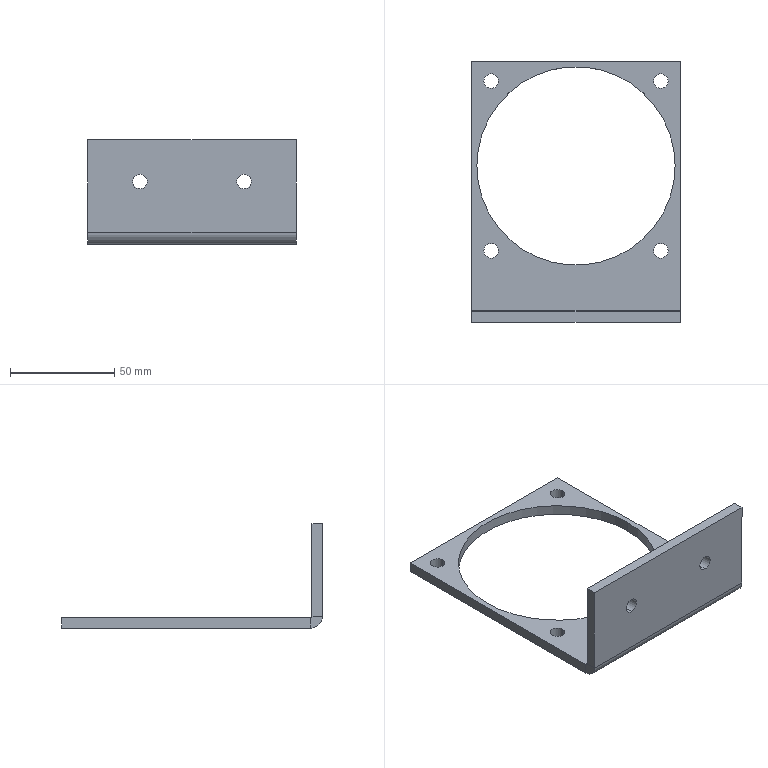Part | SolidWorks | features Cut 1, EdgeFlange 1, FlatPattern 1, ICE 1, SMBaseFlange 1, SheetMetal 1 | 1 solid | 28 faces | box 100 x 125 x 50 mm | volume 47710 mm3 | cylinder 16 | plane 12 | commonest cylinder face diameters 7 x12 95 x2 1.473 x1 11.473 x1
STEP:
#1=CARTESIAN_POINT('',(37.159,53.159,-5.));
#2=VERTEX_POINT('',#1);
#3=CARTESIAN_POINT('',(44.159,53.159,-5.));
#4=VERTEX_POINT('',#3);
#5=CARTESIAN_POINT('',(40.659,53.159,-5.));
#6=DIRECTION('',(0.,0.,1.));
#7=DIRECTION('',(1.,0.,0.));
#8=AXIS2_PLACEMENT_3D('',#5,#6,#7);
#9=CIRCLE('',#8,3.5);
#10=EDGE_CURVE('',#2,#4,#9,.T.);
#11=ORIENTED_EDGE('',*,*,#10,.F.);
#12=CARTESIAN_POINT('',(37.159,53.159,0.));
#13=VERTEX_POINT('',#12);
#14=CARTESIAN_POINT('',(37.159,53.159,-10.));
#15=DIRECTION('',(0.,0.,1.));
#16=VECTOR('',#15,1000.);
#17=LINE('',#14,#16);
#18=EDGE_CURVE('',#2,#13,#17,.T.);
#19=ORIENTED_EDGE('',*,*,#18,.T.);
#20=CARTESIAN_POINT('',(44.159,53.159,0.));
#21=VERTEX_POINT('',#20);
#22=CARTESIAN_POINT('',(40.659,53.159,0.));
#23=DIRECTION('',(0.,0.,1.));
#24=DIRECTION('',(1.,0.,0.));
#25=AXIS2_PLACEMENT_3D('',#22,#23,#24);
#26=CIRCLE('',#25,3.5);
#27=EDGE_CURVE('',#13,#21,#26,.T.);
#28=ORIENTED_EDGE('',*,*,#27,.T.);
#29=CARTESIAN_POINT('',(44.159,53.159,-10.));
#30=DIRECTION('',(0.,0.,1.));
#31=VECTOR('',#30,1000.);
#32=LINE('',#29,#31);
#33=EDGE_CURVE('',#4,#21,#32,.T.);
#34=ORIENTED_EDGE('',*,*,#33,.F.);
#35=EDGE_LOOP('',(#11,#19,#28,#34));
#36=FACE_OUTER_BOUND('',#35,.T.);
#37=CARTESIAN_POINT('',(40.659,53.159,-10.));
#38=DIRECTION('',(0.,0.,1.));
#39=DIRECTION('',(1.,0.,0.));
#40=AXIS2_PLACEMENT_3D('',#37,#38,#39);
#41=CYLINDRICAL_SURFACE('',#40,3.5);
#42=ADVANCED_FACE('',(#36),#41,.F.);
#43=CARTESIAN_POINT('',(37.159,-28.159,-5.));
#44=VERTEX_POINT('',#43);
#45=CARTESIAN_POINT('',(44.159,-28.159,-5.));
#46=VERTEX_POINT('',#45);
#47=CARTESIAN_POINT('',(40.659,-28.159,-5.));
#48=DIRECTION('',(0.,0.,1.));
#49=DIRECTION('',(1.,0.,0.));
#50=AXIS2_PLACEMENT_3D('',#47,#48,#49);
#51=CIRCLE('',#50,3.5);
#52=EDGE_CURVE('',#44,#46,#51,.T.);
#53=ORIENTED_EDGE('',*,*,#52,.F.);
#54=CARTESIAN_POINT('',(37.159,-28.159,0.));
#55=VERTEX_POINT('',#54);
#56=CARTESIAN_POINT('',(37.159,-28.159,-10.));
#57=DIRECTION('',(0.,0.,1.));
#58=VECTOR('',#57,1000.);
#59=LINE('',#56,#58);
#60=EDGE_CURVE('',#44,#55,#59,.T.);
#61=ORIENTED_EDGE('',*,*,#60,.T.);
#62=CARTESIAN_POINT('',(44.159,-28.159,0.));
#63=VERTEX_POINT('',#62);
#64=CARTESIAN_POINT('',(40.659,-28.159,0.));
#65=DIRECTION('',(0.,0.,1.));
#66=DIRECTION('',(1.,0.,0.));
#67=AXIS2_PLACEMENT_3D('',#64,#65,#66);
#68=CIRCLE('',#67,3.5);
#69=EDGE_CURVE('',#55,#63,#68,.T.);
#70=ORIENTED_EDGE('',*,*,#69,.T.);
#71=CARTESIAN_POINT('',(44.159,-28.159,-10.));
#72=DIRECTION('',(0.,0.,1.));
#73=VECTOR('',#72,1000.);
#74=LINE('',#71,#73);
#75=EDGE_CURVE('',#46,#63,#74,.T.);
#76=ORIENTED_EDGE('',*,*,#75,.F.);
#77=EDGE_LOOP('',(#53,#61,#70,#76));
#78=FACE_OUTER_BOUND('',#77,.T.);
#79=CARTESIAN_POINT('',(40.659,-28.159,-10.));
#80=DIRECTION('',(0.,0.,1.));
#81=DIRECTION('',(1.,0.,0.));
#82=AXIS2_PLACEMENT_3D('',#79,#80,#81);
#83=CYLINDRICAL_SURFACE('',#82,3.5);
#84=ADVANCED_FACE('',(#78),#83,.F.);
#85=CARTESIAN_POINT('',(-44.159,-28.159,-5.));
#86=VERTEX_POINT('',#85);
#87=CARTESIAN_POINT('',(-37.159,-28.159,-5.));
#88=VERTEX_POINT('',#87);
#89=CARTESIAN_POINT('',(-40.659,-28.159,-5.));
#90=DIRECTION('',(0.,0.,1.));
#91=DIRECTION('',(1.,0.,0.));
#92=AXIS2_PLACEMENT_3D('',#89,#90,#91);
#93=CIRCLE('',#92,3.5);
#94=EDGE_CURVE('',#86,#88,#93,.T.);
#95=ORIENTED_EDGE('',*,*,#94,.F.);
#96=CARTESIAN_POINT('',(-44.159,-28.159,0.));
#97=VERTEX_POINT('',#96);
#98=CARTESIAN_POINT('',(-44.159,-28.159,-10.));
#99=DIRECTION('',(0.,0.,1.));
#100=VECTOR('',#99,1000.);
#101=LINE('',#98,#100);
#102=EDGE_CURVE('',#86,#97,#101,.T.);
#103=ORIENTED_EDGE('',*,*,#102,.T.);
#104=CARTESIAN_POINT('',(-37.159,-28.159,0.));
#105=VERTEX_POINT('',#104);
#106=CARTESIAN_POINT('',(-40.659,-28.159,0.));
#107=DIRECTION('',(0.,0.,1.));
#108=DIRECTION('',(1.,0.,0.));
#109=AXIS2_PLACEMENT_3D('',#106,#107,#108);
#110=CIRCLE('',#109,3.5);
#111=EDGE_CURVE('',#97,#105,#110,.T.);
#112=ORIENTED_EDGE('',*,*,#111,.T.);
#113=CARTESIAN_POINT('',(-37.159,-28.159,-10.));
#114=DIRECTION('',(0.,0.,1.));
#115=VECTOR('',#114,1000.);
#116=LINE('',#113,#115);
#117=EDGE_CURVE('',#88,#105,#116,.T.);
#118=ORIENTED_EDGE('',*,*,#117,.F.);
#119=EDGE_LOOP('',(#95,#103,#112,#118));
#120=FACE_OUTER_BOUND('',#119,.T.);
#121=CARTESIAN_POINT('',(-40.659,-28.159,-10.));
#122=DIRECTION('',(0.,0.,1.));
#123=DIRECTION('',(1.,0.,0.));
#124=AXIS2_PLACEMENT_3D('',#121,#122,#123);
#125=CYLINDRICAL_SURFACE('',#124,3.5);
#126=ADVANCED_FACE('',(#120),#125,.F.);
#127=CARTESIAN_POINT('',(-44.159,53.159,-5.));
#128=VERTEX_POINT('',#127);
#129=CARTESIAN_POINT('',(-37.159,53.159,-5.));
#130=VERTEX_POINT('',#129);
#131=CARTESIAN_POINT('',(-40.659,53.159,-5.));
#132=DIRECTION('',(0.,0.,1.));
#133=DIRECTION('',(1.,0.,0.));
#134=AXIS2_PLACEMENT_3D('',#131,#132,#133);
#135=CIRCLE('',#134,3.5);
#136=EDGE_CURVE('',#128,#130,#135,.T.);
#137=ORIENTED_EDGE('',*,*,#136,.F.);
#138=CARTESIAN_POINT('',(-44.159,53.159,0.));
#139=VERTEX_POINT('',#138);
#140=CARTESIAN_POINT('',(-44.159,53.159,-10.));
#141=DIRECTION('',(0.,0.,1.));
#142=VECTOR('',#141,1000.);
#143=LINE('',#140,#142);
#144=EDGE_CURVE('',#128,#139,#143,.T.);
#145=ORIENTED_EDGE('',*,*,#144,.T.);
#146=CARTESIAN_POINT('',(-37.159,53.159,0.));
#147=VERTEX_POINT('',#146);
#148=CARTESIAN_POINT('',(-40.659,53.159,0.));
#149=DIRECTION('',(0.,0.,1.));
#150=DIRECTION('',(1.,0.,0.));
#151=AXIS2_PLACEMENT_3D('',#148,#149,#150);
#152=CIRCLE('',#151,3.5);
#153=EDGE_CURVE('',#139,#147,#152,.T.);
#154=ORIENTED_EDGE('',*,*,#153,.T.);
#155=CARTESIAN_POINT('',(-37.159,53.159,-10.));
#156=DIRECTION('',(0.,0.,1.));
#157=VECTOR('',#156,1000.);
#158=LINE('',#155,#157);
#159=EDGE_CURVE('',#130,#147,#158,.T.);
#160=ORIENTED_EDGE('',*,*,#159,.F.);
#161=EDGE_LOOP('',(#137,#145,#154,#160));
#162=FACE_OUTER_BOUND('',#161,.T.);
#163=CARTESIAN_POINT('',(-40.659,53.159,-10.));
#164=DIRECTION('',(0.,0.,1.));
#165=DIRECTION('',(1.,0.,0.));
#166=AXIS2_PLACEMENT_3D('',#163,#164,#165);
#167=CYLINDRICAL_SURFACE('',#166,3.5);
#168=ADVANCED_FACE('',(#162),#167,.F.);
#169=CARTESIAN_POINT('',(-47.5,12.5,-5.));
#170=VERTEX_POINT('',#169);
#171=CARTESIAN_POINT('',(47.5,12.5,-5.));
#172=VERTEX_POINT('',#171);
#173=CARTESIAN_POINT('',(0.,12.5,-5.));
#174=DIRECTION('',(0.,0.,1.));
#175=DIRECTION('',(1.,0.,0.));
#176=AXIS2_PLACEMENT_3D('',#173,#174,#175);
#177=CIRCLE('',#176,47.5);
#178=EDGE_CURVE('',#170,#172,#177,.T.);
#179=ORIENTED_EDGE('',*,*,#178,.F.);
#180=CARTESIAN_POINT('',(-47.5,12.5,0.));
#181=VERTEX_POINT('',#180);
#182=CARTESIAN_POINT('',(-47.5,12.5,-10.));
#183=DIRECTION('',(0.,0.,1.));
#184=VECTOR('',#183,1000.);
#185=LINE('',#182,#184);
#186=EDGE_CURVE('',#170,#181,#185,.T.);
#187=ORIENTED_EDGE('',*,*,#186,.T.);
#188=CARTESIAN_POINT('',(47.5,12.5,0.));
#189=VERTEX_POINT('',#188);
#190=CARTESIAN_POINT('',(0.,12.5,0.));
#191=DIRECTION('',(0.,0.,1.));
#192=DIRECTION('',(1.,0.,0.));
#193=AXIS2_PLACEMENT_3D('',#190,#191,#192);
#194=CIRCLE('',#193,47.5);
#195=EDGE_CURVE('',#181,#189,#194,.T.);
#196=ORIENTED_EDGE('',*,*,#195,.T.);
#197=CARTESIAN_POINT('',(47.5,12.5,-10.));
#198=DIRECTION('',(0.,0.,1.));
#199=VECTOR('',#198,1000.);
#200=LINE('',#197,#199);
#201=EDGE_CURVE('',#172,#189,#200,.T.);
#202=ORIENTED_EDGE('',*,*,#201,.F.);
#203=EDGE_LOOP('',(#179,#187,#196,#202));
#204=FACE_OUTER_BOUND('',#203,.T.);
#205=CARTESIAN_POINT('',(0.,12.5,-10.));
#206=DIRECTION('',(0.,0.,1.));
#207=DIRECTION('',(1.,0.,0.));
#208=AXIS2_PLACEMENT_3D('',#205,#206,#207);
#209=CYLINDRICAL_SURFACE('',#208,47.5);
#210=ADVANCED_FACE('',(#204),#209,.F.);
#211=CARTESIAN_POINT('',(-25.,-62.5,28.5));
#212=VERTEX_POINT('',#211);
#213=CARTESIAN_POINT('',(-25.,-62.5,21.5));
#214=VERTEX_POINT('',#213);
#215=CARTESIAN_POINT('',(-25.,-62.5,25.));
#216=DIRECTION('',(0.,-1.,0.));
#217=DIRECTION('',(0.,0.,-1.));
#218=AXIS2_PLACEMENT_3D('',#215,#216,#217);
#219=CIRCLE('',#218,3.5);
#220=EDGE_CURVE('',#212,#214,#219,.T.);
#221=ORIENTED_EDGE('',*,*,#220,.T.);
#222=CARTESIAN_POINT('',(-25.,-57.5,21.5));
#223=VERTEX_POINT('',#222);
#224=CARTESIAN_POINT('',(-25.,-67.5,21.5));
#225=DIRECTION('',(0.,1.,0.));
#226=VECTOR('',#225,1000.);
#227=LINE('',#224,#226);
#228=EDGE_CURVE('',#214,#223,#227,.T.);
#229=ORIENTED_EDGE('',*,*,#228,.T.);
#230=CARTESIAN_POINT('',(-25.,-57.5,28.5));
#231=VERTEX_POINT('',#230);
#232=CARTESIAN_POINT('',(-25.,-57.5,25.));
#233=DIRECTION('',(0.,1.,0.));
#234=DIRECTION('',(0.,0.,1.));
#235=AXIS2_PLACEMENT_3D('',#232,#233,#234);
#236=CIRCLE('',#235,3.5);
#237=EDGE_CURVE('',#223,#231,#236,.T.);
#238=ORIENTED_EDGE('',*,*,#237,.T.);
#239=CARTESIAN_POINT('',(-25.,-67.5,28.5));
#240=DIRECTION('',(0.,1.,0.));
#241=VECTOR('',#240,1000.);
#242=LINE('',#239,#241);
#243=EDGE_CURVE('',#212,#231,#242,.T.);
#244=ORIENTED_EDGE('',*,*,#243,.F.);
#245=EDGE_LOOP('',(#221,#229,#238,#244));
#246=FACE_OUTER_BOUND('',#245,.T.);
#247=CARTESIAN_POINT('',(-25.,-67.5,25.));
#248=DIRECTION('',(0.,1.,0.));
#249=DIRECTION('',(0.,0.,1.));
#250=AXIS2_PLACEMENT_3D('',#247,#248,#249);
#251=CYLINDRICAL_SURFACE('',#250,3.5);
#252=ADVANCED_FACE('',(#246),#251,.F.);
#253=CARTESIAN_POINT('',(25.,-62.5,28.5));
#254=VERTEX_POINT('',#253);
#255=CARTESIAN_POINT('',(25.,-62.5,21.5));
#256=VERTEX_POINT('',#255);
#257=CARTESIAN_POINT('',(25.,-62.5,25.));
#258=DIRECTION('',(0.,-1.,0.));
#259=DIRECTION('',(0.,0.,-1.));
#260=AXIS2_PLACEMENT_3D('',#257,#258,#259);
#261=CIRCLE('',#260,3.5);
#262=EDGE_CURVE('',#254,#256,#261,.T.);
#263=ORIENTED_EDGE('',*,*,#262,.T.);
#264=CARTESIAN_POINT('',(25.,-57.5,21.5));
#265=VERTEX_POINT('',#264);
#266=CARTESIAN_POINT('',(25.,-67.5,21.5));
#267=DIRECTION('',(0.,1.,0.));
#268=VECTOR('',#267,1000.);
#269=LINE('',#266,#268);
#270=EDGE_CURVE('',#256,#265,#269,.T.);
#271=ORIENTED_EDGE('',*,*,#270,.T.);
#272=CARTESIAN_POINT('',(25.,-57.5,28.5));
#273=VERTEX_POINT('',#272);
#274=CARTESIAN_POINT('',(25.,-57.5,25.));
#275=DIRECTION('',(0.,1.,0.));
#276=DIRECTION('',(0.,0.,-1.));
#277=AXIS2_PLACEMENT_3D('',#274,#275,#276);
#278=CIRCLE('',#277,3.5);
#279=EDGE_CURVE('',#265,#273,#278,.T.);
#280=ORIENTED_EDGE('',*,*,#279,.T.);
#281=CARTESIAN_POINT('',(25.,-67.5,28.5));
#282=DIRECTION('',(0.,1.,0.));
#283=VECTOR('',#282,1000.);
#284=LINE('',#281,#283);
#285=EDGE_CURVE('',#254,#273,#284,.T.);
#286=ORIENTED_EDGE('',*,*,#285,.F.);
#287=EDGE_LOOP('',(#263,#271,#280,#286));
#288=FACE_OUTER_BOUND('',#287,.T.);
#289=CARTESIAN_POINT('',(25.,-67.5,25.));
#290=DIRECTION('',(0.,1.,0.));
#291=DIRECTION('',(0.,0.,1.));
#292=AXIS2_PLACEMENT_3D('',#289,#290,#291);
#293=CYLINDRICAL_SURFACE('',#292,3.5);
#294=ADVANCED_FACE('',(#288),#293,.F.);
#295=CARTESIAN_POINT('',(50.,-56.763,0.));
#296=VERTEX_POINT('',#295);
#297=CARTESIAN_POINT('',(50.,62.5,0.));
#298=VERTEX_POINT('',#297);
#299=CARTESIAN_POINT('',(50.,62.5,0.));
#300=DIRECTION('',(0.,1.,0.));
#301=VECTOR('',#300,1000.);
#302=LINE('',#299,#301);
#303=EDGE_CURVE('',#296,#298,#302,.T.);
#304=ORIENTED_EDGE('',*,*,#303,.F.);
#305=CARTESIAN_POINT('',(50.,-56.763,-5.));
#306=VERTEX_POINT('',#305);
#307=CARTESIAN_POINT('',(50.,-56.763,0.));
#308=DIRECTION('',(0.,0.,-1.));
#309=VECTOR('',#308,1000.);
#310=LINE('',#307,#309);
#311=EDGE_CURVE('',#296,#306,#310,.T.);
#312=ORIENTED_EDGE('',*,*,#311,.T.);
#313=CARTESIAN_POINT('',(50.,62.5,-5.));
#314=VERTEX_POINT('',#313);
#315=CARTESIAN_POINT('',(50.,62.5,-5.));
#316=DIRECTION('',(0.,1.,0.));
#317=VECTOR('',#316,1000.);
#318=LINE('',#315,#317);
#319=EDGE_CURVE('',#306,#314,#318,.T.);
#320=ORIENTED_EDGE('',*,*,#319,.T.);
#321=CARTESIAN_POINT('',(50.,62.5,-5.));
#322=DIRECTION('',(0.,0.,1.));
#323=VECTOR('',#322,1000.);
#324=LINE('',#321,#323);
#325=EDGE_CURVE('',#314,#298,#324,.T.);
#326=ORIENTED_EDGE('',*,*,#325,.T.);
#327=EDGE_LOOP('',(#304,#312,#320,#326));
#328=FACE_OUTER_BOUND('',#327,.T.);
#329=CARTESIAN_POINT('',(50.,62.5,-5.));
#330=DIRECTION('',(1.,0.,0.));
#331=DIRECTION('',(0.,1.,0.));
#332=AXIS2_PLACEMENT_3D('',#329,#330,#331);
#333=PLANE('',#332);
#334=ADVANCED_FACE('',(#328),#333,.T.);
#335=CARTESIAN_POINT('',(40.659,53.159,-5.));
#336=DIRECTION('',(0.,0.,1.));
#337=DIRECTION('',(1.,0.,0.));
#338=AXIS2_PLACEMENT_3D('',#335,#336,#337);
#339=CIRCLE('',#338,3.5);
#340=EDGE_CURVE('',#4,#2,#339,.T.);
#341=ORIENTED_EDGE('',*,*,#340,.T.);
#342=ORIENTED_EDGE('',*,*,#10,.T.);
#343=EDGE_LOOP('',(#341,#342));
#344=FACE_BOUND('',#343,.T.);
#345=CARTESIAN_POINT('',(40.659,-28.159,-5.));
#346=DIRECTION('',(0.,0.,1.));
#347=DIRECTION('',(1.,0.,0.));
#348=AXIS2_PLACEMENT_3D('',#345,#346,#347);
#349=CIRCLE('',#348,3.5);
#350=EDGE_CURVE('',#46,#44,#349,.T.);
#351=ORIENTED_EDGE('',*,*,#350,.T.);
#352=ORIENTED_EDGE('',*,*,#52,.T.);
#353=EDGE_LOOP('',(#351,#352));
#354=FACE_BOUND('',#353,.T.);
#355=CARTESIAN_POINT('',(-40.659,-28.159,-5.));
#356=DIRECTION('',(0.,0.,1.));
#357=DIRECTION('',(1.,0.,0.));
#358=AXIS2_PLACEMENT_3D('',#355,#356,#357);
#359=CIRCLE('',#358,3.5);
#360=EDGE_CURVE('',#88,#86,#359,.T.);
#361=ORIENTED_EDGE('',*,*,#360,.T.);
#362=ORIENTED_EDGE('',*,*,#94,.T.);
#363=EDGE_LOOP('',(#361,#362));
#364=FACE_BOUND('',#363,.T.);
#365=CARTESIAN_POINT('',(-40.659,53.159,-5.));
#366=DIRECTION('',(0.,0.,1.));
#367=DIRECTION('',(1.,0.,0.));
#368=AXIS2_PLACEMENT_3D('',#365,#366,#367);
#369=CIRCLE('',#368,3.5);
#370=EDGE_CURVE('',#130,#128,#369,.T.);
#371=ORIENTED_EDGE('',*,*,#370,.T.);
#372=ORIENTED_EDGE('',*,*,#136,.T.);
#373=EDGE_LOOP('',(#371,#372));
#374=FACE_BOUND('',#373,.T.);
#375=CARTESIAN_POINT('',(0.,12.5,-5.));
#376=DIRECTION('',(0.,0.,1.));
#377=DIRECTION('',(1.,0.,0.));
#378=AXIS2_PLACEMENT_3D('',#375,#376,#377);
#379=CIRCLE('',#378,47.5);
#380=EDGE_CURVE('',#172,#170,#379,.T.);
#381=ORIENTED_EDGE('',*,*,#380,.T.);
#382=ORIENTED_EDGE('',*,*,#178,.T.);
#383=EDGE_LOOP('',(#381,#382));
#384=FACE_BOUND('',#383,.T.);
#385=CARTESIAN_POINT('',(-50.,-56.763,-5.));
#386=VERTEX_POINT('',#385);
#387=CARTESIAN_POINT('',(50.,-56.763,-5.));
#388=DIRECTION('',(-1.,0.,0.));
#389=VECTOR('',#388,1000.);
#390=LINE('',#387,#389);
#391=EDGE_CURVE('',#306,#386,#390,.T.);
#392=ORIENTED_EDGE('',*,*,#391,.T.);
#393=CARTESIAN_POINT('',(-50.,62.5,-5.));
#394=VERTEX_POINT('',#393);
#395=CARTESIAN_POINT('',(-50.,62.5,-5.));
#396=DIRECTION('',(0.,-1.,0.));
#397=VECTOR('',#396,1000.);
#398=LINE('',#395,#397);
#399=EDGE_CURVE('',#394,#386,#398,.T.);
#400=ORIENTED_EDGE('',*,*,#399,.F.);
#401=CARTESIAN_POINT('',(-50.,62.5,-5.));
#402=DIRECTION('',(-1.,0.,0.));
#403=VECTOR('',#402,1000.);
#404=LINE('',#401,#403);
#405=EDGE_CURVE('',#314,#394,#404,.T.);
#406=ORIENTED_EDGE('',*,*,#405,.F.);
#407=ORIENTED_EDGE('',*,*,#319,.F.);
#408=EDGE_LOOP('',(#392,#400,#406,#407));
#409=FACE_OUTER_BOUND('',#408,.T.);
#410=CARTESIAN_POINT('',(0.,0.,-5.));
#411=DIRECTION('',(0.,0.,1.));
#412=DIRECTION('',(1.,0.,0.));
#413=AXIS2_PLACEMENT_3D('',#410,#411,#412);
#414=PLANE('',#413);
#415=ADVANCED_FACE('',(#344,#354,#364,#374,#384,#409),#414,.F.);
#416=CARTESIAN_POINT('',(40.659,53.159,0.));
#417=DIRECTION('',(0.,0.,1.));
#418=DIRECTION('',(1.,0.,0.));
#419=AXIS2_PLACEMENT_3D('',#416,#417,#418);
#420=CIRCLE('',#419,3.5);
#421=EDGE_CURVE('',#21,#13,#420,.T.);
#422=ORIENTED_EDGE('',*,*,#421,.F.);
#423=ORIENTED_EDGE('',*,*,#27,.F.);
#424=EDGE_LOOP('',(#422,#423));
#425=FACE_BOUND('',#424,.T.);
#426=CARTESIAN_POINT('',(40.659,-28.159,0.));
#427=DIRECTION('',(0.,0.,1.));
#428=DIRECTION('',(1.,0.,0.));
#429=AXIS2_PLACEMENT_3D('',#426,#427,#428);
#430=CIRCLE('',#429,3.5);
#431=EDGE_CURVE('',#63,#55,#430,.T.);
#432=ORIENTED_EDGE('',*,*,#431,.F.);
#433=ORIENTED_EDGE('',*,*,#69,.F.);
#434=EDGE_LOOP('',(#432,#433));
#435=FACE_BOUND('',#434,.T.);
#436=CARTESIAN_POINT('',(-40.659,-28.159,0.));
#437=DIRECTION('',(0.,0.,1.));
#438=DIRECTION('',(1.,0.,0.));
#439=AXIS2_PLACEMENT_3D('',#436,#437,#438);
#440=CIRCLE('',#439,3.5);
#441=EDGE_CURVE('',#105,#97,#440,.T.);
#442=ORIENTED_EDGE('',*,*,#441,.F.);
#443=ORIENTED_EDGE('',*,*,#111,.F.);
#444=EDGE_LOOP('',(#442,#443));
#445=FACE_BOUND('',#444,.T.);
#446=CARTESIAN_POINT('',(-40.659,53.159,0.));
#447=DIRECTION('',(0.,0.,1.));
#448=DIRECTION('',(1.,0.,0.));
#449=AXIS2_PLACEMENT_3D('',#446,#447,#448);
#450=CIRCLE('',#449,3.5);
#451=EDGE_CURVE('',#147,#139,#450,.T.);
#452=ORIENTED_EDGE('',*,*,#451,.F.);
#453=ORIENTED_EDGE('',*,*,#153,.F.);
#454=EDGE_LOOP('',(#452,#453));
#455=FACE_BOUND('',#454,.T.);
#456=CARTESIAN_POINT('',(0.,12.5,0.));
#457=DIRECTION('',(0.,0.,1.));
#458=DIRECTION('',(1.,0.,0.));
#459=AXIS2_PLACEMENT_3D('',#456,#457,#458);
#460=CIRCLE('',#459,47.5);
#461=EDGE_CURVE('',#189,#181,#460,.T.);
#462=ORIENTED_EDGE('',*,*,#461,.F.);
#463=ORIENTED_EDGE('',*,*,#195,.F.);
#464=EDGE_LOOP('',(#462,#463));
#465=FACE_BOUND('',#464,.T.);
#466=CARTESIAN_POINT('',(-50.,62.5,0.));
#467=VERTEX_POINT('',#466);
#468=CARTESIAN_POINT('',(-50.,-56.763,0.));
#469=VERTEX_POINT('',#468);
#470=CARTESIAN_POINT('',(-50.,62.5,0.));
#471=DIRECTION('',(0.,-1.,0.));
#472=VECTOR('',#471,1000.);
#473=LINE('',#470,#472);
#474=EDGE_CURVE('',#467,#469,#473,.T.);
#475=ORIENTED_EDGE('',*,*,#474,.T.);
#476=CARTESIAN_POINT('',(50.,-56.763,0.));
#477=DIRECTION('',(-1.,0.,0.));
#478=VECTOR('',#477,1000.);
#479=LINE('',#476,#478);
#480=EDGE_CURVE('',#296,#469,#479,.T.);
#481=ORIENTED_EDGE('',*,*,#480,.F.);
#482=ORIENTED_EDGE('',*,*,#303,.T.);
#483=CARTESIAN_POINT('',(-50.,62.5,0.));
#484=DIRECTION('',(-1.,0.,0.));
#485=VECTOR('',#484,1000.);
#486=LINE('',#483,#485);
#487=EDGE_CURVE('',#298,#467,#486,.T.);
#488=ORIENTED_EDGE('',*,*,#487,.T.);
#489=EDGE_LOOP('',(#475,#481,#482,#488));
#490=FACE_OUTER_BOUND('',#489,.T.);
#491=CARTESIAN_POINT('',(0.,0.,0.));
#492=DIRECTION('',(0.,0.,1.));
#493=DIRECTION('',(1.,0.,0.));
#494=AXIS2_PLACEMENT_3D('',#491,#492,#493);
#495=PLANE('',#494);
#496=ADVANCED_FACE('',(#425,#435,#445,#455,#465,#490),#495,.T.);
#497=CARTESIAN_POINT('',(-50.,-56.763,0.));
#498=DIRECTION('',(0.,0.,-1.));
#499=VECTOR('',#498,1000.);
#500=LINE('',#497,#499);
#501=EDGE_CURVE('',#469,#386,#500,.T.);
#502=ORIENTED_EDGE('',*,*,#501,.F.);
#503=ORIENTED_EDGE('',*,*,#474,.F.);
#504=CARTESIAN_POINT('',(-50.,62.5,-5.));
#505=DIRECTION('',(0.,0.,1.));
#506=VECTOR('',#505,1000.);
#507=LINE('',#504,#506);
#508=EDGE_CURVE('',#394,#467,#507,.T.);
#509=ORIENTED_EDGE('',*,*,#508,.F.);
#510=ORIENTED_EDGE('',*,*,#399,.T.);
#511=EDGE_LOOP('',(#502,#503,#509,#510));
#512=FACE_OUTER_BOUND('',#511,.T.);
#513=CARTESIAN_POINT('',(-50.,62.5,-5.));
#514=DIRECTION('',(-1.,0.,0.));
#515=DIRECTION('',(0.,-1.,0.));
#516=AXIS2_PLACEMENT_3D('',#513,#514,#515);
#517=PLANE('',#516);
#518=ADVANCED_FACE('',(#512),#517,.T.);
#519=ORIENTED_EDGE('',*,*,#487,.F.);
#520=ORIENTED_EDGE('',*,*,#325,.F.);
#521=ORIENTED_EDGE('',*,*,#405,.T.);
#522=ORIENTED_EDGE('',*,*,#508,.T.);
#523=EDGE_LOOP('',(#519,#520,#521,#522));
#524=FACE_OUTER_BOUND('',#523,.T.);
#525=CARTESIAN_POINT('',(-50.,62.5,-5.));
#526=DIRECTION('',(0.,1.,0.));
#527=DIRECTION('',(0.,0.,1.));
#528=AXIS2_PLACEMENT_3D('',#525,#526,#527);
#529=PLANE('',#528);
#530=ADVANCED_FACE('',(#524),#529,.T.);
#531=CARTESIAN_POINT('',(-50.,-57.5,0.7366));
#532=VERTEX_POINT('',#531);
#533=CARTESIAN_POINT('',(-50.,-62.5,0.7366));
#534=VERTEX_POINT('',#533);
#535=CARTESIAN_POINT('',(-50.,-62.5,0.7366));
#536=DIRECTION('',(0.,-1.,0.));
#537=VECTOR('',#536,1000.);
#538=LINE('',#535,#537);
#539=EDGE_CURVE('',#532,#534,#538,.T.);
#540=ORIENTED_EDGE('',*,*,#539,.F.);
#541=CARTESIAN_POINT('',(-50.,-56.763,0.7366));
#542=DIRECTION('',(-1.,0.,0.));
#543=DIRECTION('',(0.,0.,-1.));
#544=AXIS2_PLACEMENT_3D('',#541,#542,#543);
#545=CIRCLE('',#544,0.7366);
#546=EDGE_CURVE('',#469,#532,#545,.T.);
#547=ORIENTED_EDGE('',*,*,#546,.F.);
#548=ORIENTED_EDGE('',*,*,#501,.T.);
#549=CARTESIAN_POINT('',(-50.,-56.763,0.7366));
#550=DIRECTION('',(-1.,0.,0.));
#551=DIRECTION('',(0.,0.,-1.));
#552=AXIS2_PLACEMENT_3D('',#549,#550,#551);
#553=CIRCLE('',#552,5.737);
#554=EDGE_CURVE('',#386,#534,#553,.T.);
#555=ORIENTED_EDGE('',*,*,#554,.T.);
#556=EDGE_LOOP('',(#540,#547,#548,#555));
#557=FACE_OUTER_BOUND('',#556,.T.);
#558=CARTESIAN_POINT('',(-50.,-56.763,0.7366));
#559=DIRECTION('',(-1.,0.,0.));
#560=DIRECTION('',(0.,0.,1.));
#561=AXIS2_PLACEMENT_3D('',#558,#559,#560);
#562=PLANE('',#561);
#563=ADVANCED_FACE('',(#557),#562,.T.);
#564=CARTESIAN_POINT('',(50.,-57.5,0.7366));
#565=VERTEX_POINT('',#564);
#566=CARTESIAN_POINT('',(50.,-56.763,0.7366));
#567=DIRECTION('',(1.,0.,0.));
#568=DIRECTION('',(0.,0.,-1.));
#569=AXIS2_PLACEMENT_3D('',#566,#567,#568);
#570=CIRCLE('',#569,0.7366);
#571=EDGE_CURVE('',#565,#296,#570,.T.);
#572=ORIENTED_EDGE('',*,*,#571,.F.);
#573=CARTESIAN_POINT('',(50.,-62.5,0.7366));
#574=VERTEX_POINT('',#573);
#575=CARTESIAN_POINT('',(50.,-57.5,0.7366));
#576=DIRECTION('',(0.,-1.,0.));
#577=VECTOR('',#576,1000.);
#578=LINE('',#575,#577);
#579=EDGE_CURVE('',#565,#574,#578,.T.);
#580=ORIENTED_EDGE('',*,*,#579,.T.);
#581=CARTESIAN_POINT('',(50.,-56.763,0.7366));
#582=DIRECTION('',(1.,0.,0.));
#583=DIRECTION('',(0.,0.,-1.));
#584=AXIS2_PLACEMENT_3D('',#581,#582,#583);
#585=CIRCLE('',#584,5.737);
#586=EDGE_CURVE('',#574,#306,#585,.T.);
#587=ORIENTED_EDGE('',*,*,#586,.T.);
#588=ORIENTED_EDGE('',*,*,#311,.F.);
#589=EDGE_LOOP('',(#572,#580,#587,#588));
#590=FACE_OUTER_BOUND('',#589,.T.);
#591=CARTESIAN_POINT('',(50.,-56.763,0.7366));
#592=DIRECTION('',(-1.,0.,0.));
#593=DIRECTION('',(0.,0.,1.));
#594=AXIS2_PLACEMENT_3D('',#591,#592,#593);
#595=PLANE('',#594);
#596=ADVANCED_FACE('',(#590),#595,.F.);
#597=ORIENTED_EDGE('',*,*,#391,.F.);
#598=ORIENTED_EDGE('',*,*,#586,.F.);
#599=CARTESIAN_POINT('',(0.,-62.5,0.7366));
#600=DIRECTION('',(1.,0.,0.));
#601=VECTOR('',#600,1000.);
#602=LINE('',#599,#601);
#603=EDGE_CURVE('',#534,#574,#602,.T.);
#604=ORIENTED_EDGE('',*,*,#603,.F.);
#605=ORIENTED_EDGE('',*,*,#554,.F.);
#606=EDGE_LOOP('',(#597,#598,#604,#605));
#607=FACE_OUTER_BOUND('',#606,.T.);
#608=CARTESIAN_POINT('',(50.,-56.763,0.7366));
#609=DIRECTION('',(1.,0.,0.));
#610=DIRECTION('',(0.,-1.,0.));
#611=AXIS2_PLACEMENT_3D('',#608,#609,#610);
#612=CYLINDRICAL_SURFACE('',#611,5.737);
#613=ADVANCED_FACE('',(#607),#612,.T.);
#614=ORIENTED_EDGE('',*,*,#480,.T.);
#615=ORIENTED_EDGE('',*,*,#546,.T.);
#616=CARTESIAN_POINT('',(-50.,-57.5,0.7366));
#617=DIRECTION('',(1.,0.,0.));
#618=VECTOR('',#617,1000.);
#619=LINE('',#616,#618);
#620=EDGE_CURVE('',#532,#565,#619,.T.);
#621=ORIENTED_EDGE('',*,*,#620,.T.);
#622=ORIENTED_EDGE('',*,*,#571,.T.);
#623=EDGE_LOOP('',(#614,#615,#621,#622));
#624=FACE_OUTER_BOUND('',#623,.T.);
#625=CARTESIAN_POINT('',(50.,-56.763,0.7366));
#626=DIRECTION('',(1.,0.,0.));
#627=DIRECTION('',(0.,-1.,0.));
#628=AXIS2_PLACEMENT_3D('',#625,#626,#627);
#629=CYLINDRICAL_SURFACE('',#628,0.7366);
#630=ADVANCED_FACE('',(#624),#629,.F.);
#631=CARTESIAN_POINT('',(50.,-62.5,45.));
#632=VERTEX_POINT('',#631);
#633=CARTESIAN_POINT('',(50.,-62.5,0.));
#634=DIRECTION('',(0.,0.,-1.));
#635=VECTOR('',#634,1000.);
#636=LINE('',#633,#635);
#637=EDGE_CURVE('',#632,#574,#636,.T.);
#638=ORIENTED_EDGE('',*,*,#637,.T.);
#639=ORIENTED_EDGE('',*,*,#579,.F.);
#640=CARTESIAN_POINT('',(50.,-57.5,45.));
#641=VERTEX_POINT('',#640);
#642=CARTESIAN_POINT('',(50.,-57.5,0.));
#643=DIRECTION('',(0.,0.,-1.));
#644=VECTOR('',#643,1000.);
#645=LINE('',#642,#644);
#646=EDGE_CURVE('',#641,#565,#645,.T.);
#647=ORIENTED_EDGE('',*,*,#646,.F.);
#648=CARTESIAN_POINT('',(50.,-62.5,45.));
#649=DIRECTION('',(0.,1.,0.));
#650=VECTOR('',#649,1000.);
#651=LINE('',#648,#650);
#652=EDGE_CURVE('',#632,#641,#651,.T.);
#653=ORIENTED_EDGE('',*,*,#652,.F.);
#654=EDGE_LOOP('',(#638,#639,#647,#653));
#655=FACE_OUTER_BOUND('',#654,.T.);
#656=CARTESIAN_POINT('',(50.,-62.5,0.));
#657=DIRECTION('',(1.,0.,0.));
#658=DIRECTION('',(0.,0.,-1.));
#659=AXIS2_PLACEMENT_3D('',#656,#657,#658);
#660=PLANE('',#659);
#661=ADVANCED_FACE('',(#655),#660,.T.);
#662=CARTESIAN_POINT('',(-50.,-57.5,45.));
#663=VERTEX_POINT('',#662);
#664=CARTESIAN_POINT('',(-50.,-57.5,0.));
#665=DIRECTION('',(0.,0.,1.));
#666=VECTOR('',#665,1000.);
#667=LINE('',#664,#666);
#668=EDGE_CURVE('',#532,#663,#667,.T.);
#669=ORIENTED_EDGE('',*,*,#668,.F.);
#670=ORIENTED_EDGE('',*,*,#539,.T.);
#671=CARTESIAN_POINT('',(-50.,-62.5,45.));
#672=VERTEX_POINT('',#671);
#673=CARTESIAN_POINT('',(-50.,-62.5,45.));
#674=DIRECTION('',(0.,0.,1.));
#675=VECTOR('',#674,1000.);
#676=LINE('',#673,#675);
#677=EDGE_CURVE('',#534,#672,#676,.T.);
#678=ORIENTED_EDGE('',*,*,#677,.T.);
#679=CARTESIAN_POINT('',(-50.,-62.5,45.));
#680=DIRECTION('',(0.,1.,0.));
#681=VECTOR('',#680,1000.);
#682=LINE('',#679,#681);
#683=EDGE_CURVE('',#672,#663,#682,.T.);
#684=ORIENTED_EDGE('',*,*,#683,.T.);
#685=EDGE_LOOP('',(#669,#670,#678,#684));
#686=FACE_OUTER_BOUND('',#685,.T.);
#687=CARTESIAN_POINT('',(-50.,-62.5,45.));
#688=DIRECTION('',(-1.,0.,0.));
#689=DIRECTION('',(0.,0.,1.));
#690=AXIS2_PLACEMENT_3D('',#687,#688,#689);
#691=PLANE('',#690);
#692=ADVANCED_FACE('',(#686),#691,.T.);
#693=ORIENTED_EDGE('',*,*,#220,.F.);
#694=CARTESIAN_POINT('',(-25.,-62.5,25.));
#695=DIRECTION('',(0.,-1.,0.));
#696=DIRECTION('',(0.,0.,-1.));
#697=AXIS2_PLACEMENT_3D('',#694,#695,#696);
#698=CIRCLE('',#697,3.5);
#699=EDGE_CURVE('',#214,#212,#698,.T.);
#700=ORIENTED_EDGE('',*,*,#699,.F.);
#701=EDGE_LOOP('',(#693,#700));
#702=FACE_BOUND('',#701,.T.);
#703=ORIENTED_EDGE('',*,*,#262,.F.);
#704=CARTESIAN_POINT('',(25.,-62.5,25.));
#705=DIRECTION('',(0.,-1.,0.));
#706=DIRECTION('',(0.,0.,-1.));
#707=AXIS2_PLACEMENT_3D('',#704,#705,#706);
#708=CIRCLE('',#707,3.5);
#709=EDGE_CURVE('',#256,#254,#708,.T.);
#710=ORIENTED_EDGE('',*,*,#709,.F.);
#711=EDGE_LOOP('',(#703,#710));
#712=FACE_BOUND('',#711,.T.);
#713=ORIENTED_EDGE('',*,*,#677,.F.);
#714=ORIENTED_EDGE('',*,*,#603,.T.);
#715=ORIENTED_EDGE('',*,*,#637,.F.);
#716=CARTESIAN_POINT('',(50.,-62.5,45.));
#717=DIRECTION('',(1.,0.,0.));
#718=VECTOR('',#717,1000.);
#719=LINE('',#716,#718);
#720=EDGE_CURVE('',#672,#632,#719,.T.);
#721=ORIENTED_EDGE('',*,*,#720,.F.);
#722=EDGE_LOOP('',(#713,#714,#715,#721));
#723=FACE_OUTER_BOUND('',#722,.T.);
#724=CARTESIAN_POINT('',(0.,-62.5,0.));
#725=DIRECTION('',(0.,-1.,0.));
#726=DIRECTION('',(0.,0.,-1.));
#727=AXIS2_PLACEMENT_3D('',#724,#725,#726);
#728=PLANE('',#727);
#729=ADVANCED_FACE('',(#702,#712,#723),#728,.T.);
#730=CARTESIAN_POINT('',(-25.,-57.5,25.));
#731=DIRECTION('',(0.,1.,0.));
#732=DIRECTION('',(0.,0.,1.));
#733=AXIS2_PLACEMENT_3D('',#730,#731,#732);
#734=CIRCLE('',#733,3.5);
#735=EDGE_CURVE('',#231,#223,#734,.T.);
#736=ORIENTED_EDGE('',*,*,#735,.F.);
#737=ORIENTED_EDGE('',*,*,#237,.F.);
#738=EDGE_LOOP('',(#736,#737));
#739=FACE_BOUND('',#738,.T.);
#740=CARTESIAN_POINT('',(25.,-57.5,25.));
#741=DIRECTION('',(0.,1.,0.));
#742=DIRECTION('',(0.,0.,-1.));
#743=AXIS2_PLACEMENT_3D('',#740,#741,#742);
#744=CIRCLE('',#743,3.5);
#745=EDGE_CURVE('',#273,#265,#744,.T.);
#746=ORIENTED_EDGE('',*,*,#745,.F.);
#747=ORIENTED_EDGE('',*,*,#279,.F.);
#748=EDGE_LOOP('',(#746,#747));
#749=FACE_BOUND('',#748,.T.);
#750=ORIENTED_EDGE('',*,*,#620,.F.);
#751=ORIENTED_EDGE('',*,*,#668,.T.);
#752=CARTESIAN_POINT('',(0.,-57.5,45.));
#753=DIRECTION('',(1.,0.,0.));
#754=VECTOR('',#753,1000.);
#755=LINE('',#752,#754);
#756=EDGE_CURVE('',#663,#641,#755,.T.);
#757=ORIENTED_EDGE('',*,*,#756,.T.);
#758=ORIENTED_EDGE('',*,*,#646,.T.);
#759=EDGE_LOOP('',(#750,#751,#757,#758));
#760=FACE_OUTER_BOUND('',#759,.T.);
#761=CARTESIAN_POINT('',(0.,-57.5,0.));
#762=DIRECTION('',(0.,-1.,0.));
#763=DIRECTION('',(0.,0.,-1.));
#764=AXIS2_PLACEMENT_3D('',#761,#762,#763);
#765=PLANE('',#764);
#766=ADVANCED_FACE('',(#739,#749,#760),#765,.F.);
#767=ORIENTED_EDGE('',*,*,#756,.F.);
#768=ORIENTED_EDGE('',*,*,#683,.F.);
#769=ORIENTED_EDGE('',*,*,#720,.T.);
#770=ORIENTED_EDGE('',*,*,#652,.T.);
#771=EDGE_LOOP('',(#767,#768,#769,#770));
#772=FACE_OUTER_BOUND('',#771,.T.);
#773=CARTESIAN_POINT('',(50.,-62.5,45.));
#774=DIRECTION('',(0.,0.,1.));
#775=DIRECTION('',(0.,-1.,0.));
#776=AXIS2_PLACEMENT_3D('',#773,#774,#775);
#777=PLANE('',#776);
#778=ADVANCED_FACE('',(#772),#777,.T.);
#779=ORIENTED_EDGE('',*,*,#270,.F.);
#780=ORIENTED_EDGE('',*,*,#709,.T.);
#781=ORIENTED_EDGE('',*,*,#285,.T.);
#782=ORIENTED_EDGE('',*,*,#745,.T.);
#783=EDGE_LOOP('',(#779,#780,#781,#782));
#784=FACE_OUTER_BOUND('',#783,.T.);
#785=CARTESIAN_POINT('',(25.,-67.5,25.));
#786=DIRECTION('',(0.,1.,0.));
#787=DIRECTION('',(0.,0.,1.));
#788=AXIS2_PLACEMENT_3D('',#785,#786,#787);
#789=CYLINDRICAL_SURFACE('',#788,3.5);
#790=ADVANCED_FACE('',(#784),#789,.F.);
#791=ORIENTED_EDGE('',*,*,#228,.F.);
#792=ORIENTED_EDGE('',*,*,#699,.T.);
#793=ORIENTED_EDGE('',*,*,#243,.T.);
#794=ORIENTED_EDGE('',*,*,#735,.T.);
#795=EDGE_LOOP('',(#791,#792,#793,#794));
#796=FACE_OUTER_BOUND('',#795,.T.);
#797=CARTESIAN_POINT('',(-25.,-67.5,25.));
#798=DIRECTION('',(0.,1.,0.));
#799=DIRECTION('',(0.,0.,1.));
#800=AXIS2_PLACEMENT_3D('',#797,#798,#799);
#801=CYLINDRICAL_SURFACE('',#800,3.5);
#802=ADVANCED_FACE('',(#796),#801,.F.);
#803=ORIENTED_EDGE('',*,*,#186,.F.);
#804=ORIENTED_EDGE('',*,*,#380,.F.);
#805=ORIENTED_EDGE('',*,*,#201,.T.);
#806=ORIENTED_EDGE('',*,*,#461,.T.);
#807=EDGE_LOOP('',(#803,#804,#805,#806));
#808=FACE_OUTER_BOUND('',#807,.T.);
#809=CARTESIAN_POINT('',(0.,12.5,-10.));
#810=DIRECTION('',(0.,0.,1.));
#811=DIRECTION('',(1.,0.,0.));
#812=AXIS2_PLACEMENT_3D('',#809,#810,#811);
#813=CYLINDRICAL_SURFACE('',#812,47.5);
#814=ADVANCED_FACE('',(#808),#813,.F.);
#815=ORIENTED_EDGE('',*,*,#144,.F.);
#816=ORIENTED_EDGE('',*,*,#370,.F.);
#817=ORIENTED_EDGE('',*,*,#159,.T.);
#818=ORIENTED_EDGE('',*,*,#451,.T.);
#819=EDGE_LOOP('',(#815,#816,#817,#818));
#820=FACE_OUTER_BOUND('',#819,.T.);
#821=CARTESIAN_POINT('',(-40.659,53.159,-10.));
#822=DIRECTION('',(0.,0.,1.));
#823=DIRECTION('',(1.,0.,0.));
#824=AXIS2_PLACEMENT_3D('',#821,#822,#823);
#825=CYLINDRICAL_SURFACE('',#824,3.5);
#826=ADVANCED_FACE('',(#820),#825,.F.);
#827=ORIENTED_EDGE('',*,*,#102,.F.);
#828=ORIENTED_EDGE('',*,*,#360,.F.);
#829=ORIENTED_EDGE('',*,*,#117,.T.);
#830=ORIENTED_EDGE('',*,*,#441,.T.);
#831=EDGE_LOOP('',(#827,#828,#829,#830));
#832=FACE_OUTER_BOUND('',#831,.T.);
#833=CARTESIAN_POINT('',(-40.659,-28.159,-10.));
#834=DIRECTION('',(0.,0.,1.));
#835=DIRECTION('',(1.,0.,0.));
#836=AXIS2_PLACEMENT_3D('',#833,#834,#835);
#837=CYLINDRICAL_SURFACE('',#836,3.5);
#838=ADVANCED_FACE('',(#832),#837,.F.);
#839=ORIENTED_EDGE('',*,*,#60,.F.);
#840=ORIENTED_EDGE('',*,*,#350,.F.);
#841=ORIENTED_EDGE('',*,*,#75,.T.);
#842=ORIENTED_EDGE('',*,*,#431,.T.);
#843=EDGE_LOOP('',(#839,#840,#841,#842));
#844=FACE_OUTER_BOUND('',#843,.T.);
#845=CARTESIAN_POINT('',(40.659,-28.159,-10.));
#846=DIRECTION('',(0.,0.,1.));
#847=DIRECTION('',(1.,0.,0.));
#848=AXIS2_PLACEMENT_3D('',#845,#846,#847);
#849=CYLINDRICAL_SURFACE('',#848,3.5);
#850=ADVANCED_FACE('',(#844),#849,.F.);
#851=ORIENTED_EDGE('',*,*,#18,.F.);
#852=ORIENTED_EDGE('',*,*,#340,.F.);
#853=ORIENTED_EDGE('',*,*,#33,.T.);
#854=ORIENTED_EDGE('',*,*,#421,.T.);
#855=EDGE_LOOP('',(#851,#852,#853,#854));
#856=FACE_OUTER_BOUND('',#855,.T.);
#857=CARTESIAN_POINT('',(40.659,53.159,-10.));
#858=DIRECTION('',(0.,0.,1.));
#859=DIRECTION('',(1.,0.,0.));
#860=AXIS2_PLACEMENT_3D('',#857,#858,#859);
#861=CYLINDRICAL_SURFACE('',#860,3.5);
#862=ADVANCED_FACE('',(#856),#861,.F.);
#863=CLOSED_SHELL('',(#42,#84,#126,#168,#210,#252,#294,#334,#415,#496,#518,#530,#563,#596,#613,#630,#661,#692,#729,#766,#778,#790,#802,#814,#826,#838,#850,#862));
#864=MANIFOLD_SOLID_BREP('',#863);
#865=CARTESIAN_POINT('',(0.,0.,0.));
#866=DIRECTION('',(0.,0.,1.));
#867=DIRECTION('',(1.,0.,0.));
#868=AXIS2_PLACEMENT_3D('',#865,#866,#867);
#869=(LENGTH_UNIT()NAMED_UNIT(*)SI_UNIT(.MILLI.,.METRE.));
#870=UNCERTAINTY_MEASURE_WITH_UNIT(LENGTH_MEASURE(0.00001),#869,'','');
#871=(NAMED_UNIT(*)PLANE_ANGLE_UNIT()SI_UNIT($,.RADIAN.));
#872=(NAMED_UNIT(*)SI_UNIT($,.STERADIAN.)SOLID_ANGLE_UNIT());
#873=(GEOMETRIC_REPRESENTATION_CONTEXT(3)GLOBAL_UNCERTAINTY_ASSIGNED_CONTEXT((#870))GLOBAL_UNIT_ASSIGNED_CONTEXT((#869,#871,#872))REPRESENTATION_CONTEXT('',''));
#874=ADVANCED_BREP_SHAPE_REPRESENTATION('',(#864,#868),#873);